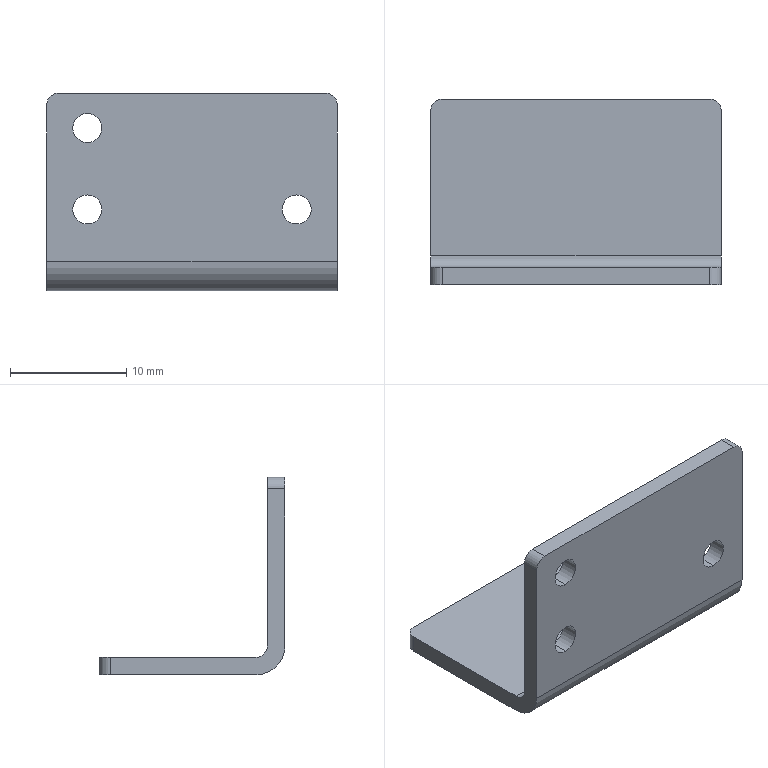Part | SolidWorks | features BaseBody 1 | 1 solid | 20 faces | box 25 x 16 x 17 mm | volume 1130 mm3 | cylinder 12 | plane 8 | commonest cylinder face diameters 2.5 x6 2 x5 5 x1
STEP:
#1=CARTESIAN_POINT('',(100.5,20.,73.25));
#2=VERTEX_POINT('',#1);
#3=CARTESIAN_POINT('',(100.5,20.,75.75));
#4=VERTEX_POINT('',#3);
#5=CARTESIAN_POINT('',(100.5,20.,74.5));
#6=DIRECTION('',(0.,1.,0.));
#7=DIRECTION('',(0.,0.,1.));
#8=AXIS2_PLACEMENT_3D('',#5,#6,#7);
#9=CIRCLE('',#8,1.25);
#10=EDGE_CURVE('',#2,#4,#9,.T.);
#11=ORIENTED_EDGE('',*,*,#10,.F.);
#12=CARTESIAN_POINT('',(100.5,21.5,73.25));
#13=VERTEX_POINT('',#12);
#14=CARTESIAN_POINT('',(100.5,46.5,73.25));
#15=DIRECTION('',(0.,1.,0.));
#16=VECTOR('',#15,1000.);
#17=LINE('',#14,#16);
#18=EDGE_CURVE('',#2,#13,#17,.T.);
#19=ORIENTED_EDGE('',*,*,#18,.T.);
#20=CARTESIAN_POINT('',(100.5,21.5,75.75));
#21=VERTEX_POINT('',#20);
#22=CARTESIAN_POINT('',(100.5,21.5,74.5));
#23=DIRECTION('',(0.,1.,0.));
#24=DIRECTION('',(0.,0.,1.));
#25=AXIS2_PLACEMENT_3D('',#22,#23,#24);
#26=CIRCLE('',#25,1.25);
#27=EDGE_CURVE('',#13,#21,#26,.T.);
#28=ORIENTED_EDGE('',*,*,#27,.T.);
#29=CARTESIAN_POINT('',(100.5,46.5,75.75));
#30=DIRECTION('',(0.,1.,0.));
#31=VECTOR('',#30,1000.);
#32=LINE('',#29,#31);
#33=EDGE_CURVE('',#4,#21,#32,.T.);
#34=ORIENTED_EDGE('',*,*,#33,.F.);
#35=EDGE_LOOP('',(#11,#19,#28,#34));
#36=FACE_OUTER_BOUND('',#35,.T.);
#37=CARTESIAN_POINT('',(100.5,46.5,74.5));
#38=DIRECTION('',(0.,1.,0.));
#39=DIRECTION('',(0.,0.,1.));
#40=AXIS2_PLACEMENT_3D('',#37,#38,#39);
#41=CYLINDRICAL_SURFACE('',#40,1.25);
#42=ADVANCED_FACE('',(#36),#41,.F.);
#43=CARTESIAN_POINT('',(118.5,20.,73.25));
#44=VERTEX_POINT('',#43);
#45=CARTESIAN_POINT('',(118.5,20.,75.75));
#46=VERTEX_POINT('',#45);
#47=CARTESIAN_POINT('',(118.5,20.,74.5));
#48=DIRECTION('',(0.,1.,0.));
#49=DIRECTION('',(0.,0.,1.));
#50=AXIS2_PLACEMENT_3D('',#47,#48,#49);
#51=CIRCLE('',#50,1.25);
#52=EDGE_CURVE('',#44,#46,#51,.T.);
#53=ORIENTED_EDGE('',*,*,#52,.F.);
#54=CARTESIAN_POINT('',(118.5,21.5,73.25));
#55=VERTEX_POINT('',#54);
#56=CARTESIAN_POINT('',(118.5,46.5,73.25));
#57=DIRECTION('',(0.,1.,0.));
#58=VECTOR('',#57,1000.);
#59=LINE('',#56,#58);
#60=EDGE_CURVE('',#44,#55,#59,.T.);
#61=ORIENTED_EDGE('',*,*,#60,.T.);
#62=CARTESIAN_POINT('',(118.5,21.5,75.75));
#63=VERTEX_POINT('',#62);
#64=CARTESIAN_POINT('',(118.5,21.5,74.5));
#65=DIRECTION('',(0.,1.,0.));
#66=DIRECTION('',(0.,0.,1.));
#67=AXIS2_PLACEMENT_3D('',#64,#65,#66);
#68=CIRCLE('',#67,1.25);
#69=EDGE_CURVE('',#55,#63,#68,.T.);
#70=ORIENTED_EDGE('',*,*,#69,.T.);
#71=CARTESIAN_POINT('',(118.5,46.5,75.75));
#72=DIRECTION('',(0.,1.,0.));
#73=VECTOR('',#72,1000.);
#74=LINE('',#71,#73);
#75=EDGE_CURVE('',#46,#63,#74,.T.);
#76=ORIENTED_EDGE('',*,*,#75,.F.);
#77=EDGE_LOOP('',(#53,#61,#70,#76));
#78=FACE_OUTER_BOUND('',#77,.T.);
#79=CARTESIAN_POINT('',(118.5,46.5,74.5));
#80=DIRECTION('',(0.,1.,0.));
#81=DIRECTION('',(0.,0.,1.));
#82=AXIS2_PLACEMENT_3D('',#79,#80,#81);
#83=CYLINDRICAL_SURFACE('',#82,1.25);
#84=ADVANCED_FACE('',(#78),#83,.F.);
#85=CARTESIAN_POINT('',(100.5,20.,80.25));
#86=VERTEX_POINT('',#85);
#87=CARTESIAN_POINT('',(100.5,20.,82.75));
#88=VERTEX_POINT('',#87);
#89=CARTESIAN_POINT('',(100.5,20.,81.5));
#90=DIRECTION('',(0.,1.,0.));
#91=DIRECTION('',(0.,0.,1.));
#92=AXIS2_PLACEMENT_3D('',#89,#90,#91);
#93=CIRCLE('',#92,1.25);
#94=EDGE_CURVE('',#86,#88,#93,.T.);
#95=ORIENTED_EDGE('',*,*,#94,.F.);
#96=CARTESIAN_POINT('',(100.5,21.5,80.25));
#97=VERTEX_POINT('',#96);
#98=CARTESIAN_POINT('',(100.5,46.5,80.25));
#99=DIRECTION('',(0.,1.,0.));
#100=VECTOR('',#99,1000.);
#101=LINE('',#98,#100);
#102=EDGE_CURVE('',#86,#97,#101,.T.);
#103=ORIENTED_EDGE('',*,*,#102,.T.);
#104=CARTESIAN_POINT('',(100.5,21.5,82.75));
#105=VERTEX_POINT('',#104);
#106=CARTESIAN_POINT('',(100.5,21.5,81.5));
#107=DIRECTION('',(0.,1.,0.));
#108=DIRECTION('',(0.,0.,1.));
#109=AXIS2_PLACEMENT_3D('',#106,#107,#108);
#110=CIRCLE('',#109,1.25);
#111=EDGE_CURVE('',#97,#105,#110,.T.);
#112=ORIENTED_EDGE('',*,*,#111,.T.);
#113=CARTESIAN_POINT('',(100.5,46.5,82.75));
#114=DIRECTION('',(0.,1.,0.));
#115=VECTOR('',#114,1000.);
#116=LINE('',#113,#115);
#117=EDGE_CURVE('',#88,#105,#116,.T.);
#118=ORIENTED_EDGE('',*,*,#117,.F.);
#119=EDGE_LOOP('',(#95,#103,#112,#118));
#120=FACE_OUTER_BOUND('',#119,.T.);
#121=CARTESIAN_POINT('',(100.5,46.5,81.5));
#122=DIRECTION('',(0.,1.,0.));
#123=DIRECTION('',(0.,0.,1.));
#124=AXIS2_PLACEMENT_3D('',#121,#122,#123);
#125=CYLINDRICAL_SURFACE('',#124,1.25);
#126=ADVANCED_FACE('',(#120),#125,.F.);
#127=CARTESIAN_POINT('',(122.,21.5,83.5));
#128=VERTEX_POINT('',#127);
#129=CARTESIAN_POINT('',(121.,21.5,84.5));
#130=VERTEX_POINT('',#129);
#131=CARTESIAN_POINT('',(121.,21.5,83.5));
#132=DIRECTION('',(0.,-1.,0.));
#133=DIRECTION('',(0.,0.,-1.));
#134=AXIS2_PLACEMENT_3D('',#131,#132,#133);
#135=CIRCLE('',#134,1.);
#136=EDGE_CURVE('',#128,#130,#135,.T.);
#137=ORIENTED_EDGE('',*,*,#136,.F.);
#138=CARTESIAN_POINT('',(122.,21.5,70.));
#139=VERTEX_POINT('',#138);
#140=CARTESIAN_POINT('',(122.,21.5,70.));
#141=DIRECTION('',(0.,0.,1.));
#142=VECTOR('',#141,1000.);
#143=LINE('',#140,#142);
#144=EDGE_CURVE('',#139,#128,#143,.T.);
#145=ORIENTED_EDGE('',*,*,#144,.F.);
#146=CARTESIAN_POINT('',(97.,21.5,70.));
#147=VERTEX_POINT('',#146);
#148=CARTESIAN_POINT('',(122.,21.5,70.));
#149=DIRECTION('',(1.,0.,0.));
#150=VECTOR('',#149,1000.);
#151=LINE('',#148,#150);
#152=EDGE_CURVE('',#147,#139,#151,.T.);
#153=ORIENTED_EDGE('',*,*,#152,.F.);
#154=CARTESIAN_POINT('',(97.,21.5,83.5));
#155=VERTEX_POINT('',#154);
#156=CARTESIAN_POINT('',(97.,21.5,70.));
#157=DIRECTION('',(0.,0.,-1.));
#158=VECTOR('',#157,1000.);
#159=LINE('',#156,#158);
#160=EDGE_CURVE('',#155,#147,#159,.T.);
#161=ORIENTED_EDGE('',*,*,#160,.F.);
#162=CARTESIAN_POINT('',(98.,21.5,84.5));
#163=VERTEX_POINT('',#162);
#164=CARTESIAN_POINT('',(98.,21.5,83.5));
#165=DIRECTION('',(0.,-1.,0.));
#166=DIRECTION('',(0.,0.,1.));
#167=AXIS2_PLACEMENT_3D('',#164,#165,#166);
#168=CIRCLE('',#167,1.);
#169=EDGE_CURVE('',#163,#155,#168,.T.);
#170=ORIENTED_EDGE('',*,*,#169,.F.);
#171=CARTESIAN_POINT('',(122.,21.5,84.5));
#172=DIRECTION('',(-1.,0.,0.));
#173=VECTOR('',#172,1000.);
#174=LINE('',#171,#173);
#175=EDGE_CURVE('',#130,#163,#174,.T.);
#176=ORIENTED_EDGE('',*,*,#175,.F.);
#177=EDGE_LOOP('',(#137,#145,#153,#161,#170,#176));
#178=FACE_OUTER_BOUND('',#177,.T.);
#179=CARTESIAN_POINT('',(100.5,21.5,74.5));
#180=DIRECTION('',(0.,1.,0.));
#181=DIRECTION('',(0.,0.,1.));
#182=AXIS2_PLACEMENT_3D('',#179,#180,#181);
#183=CIRCLE('',#182,1.25);
#184=EDGE_CURVE('',#21,#13,#183,.T.);
#185=ORIENTED_EDGE('',*,*,#184,.F.);
#186=ORIENTED_EDGE('',*,*,#27,.F.);
#187=EDGE_LOOP('',(#185,#186));
#188=FACE_BOUND('',#187,.T.);
#189=CARTESIAN_POINT('',(118.5,21.5,74.5));
#190=DIRECTION('',(0.,1.,0.));
#191=DIRECTION('',(0.,0.,1.));
#192=AXIS2_PLACEMENT_3D('',#189,#190,#191);
#193=CIRCLE('',#192,1.25);
#194=EDGE_CURVE('',#63,#55,#193,.T.);
#195=ORIENTED_EDGE('',*,*,#194,.F.);
#196=ORIENTED_EDGE('',*,*,#69,.F.);
#197=EDGE_LOOP('',(#195,#196));
#198=FACE_BOUND('',#197,.T.);
#199=CARTESIAN_POINT('',(100.5,21.5,81.5));
#200=DIRECTION('',(0.,1.,0.));
#201=DIRECTION('',(0.,0.,1.));
#202=AXIS2_PLACEMENT_3D('',#199,#200,#201);
#203=CIRCLE('',#202,1.25);
#204=EDGE_CURVE('',#105,#97,#203,.T.);
#205=ORIENTED_EDGE('',*,*,#204,.F.);
#206=ORIENTED_EDGE('',*,*,#111,.F.);
#207=EDGE_LOOP('',(#205,#206));
#208=FACE_BOUND('',#207,.T.);
#209=CARTESIAN_POINT('',(122.,21.5,70.));
#210=DIRECTION('',(0.,-1.,0.));
#211=DIRECTION('',(0.,0.,-1.));
#212=AXIS2_PLACEMENT_3D('',#209,#210,#211);
#213=PLANE('',#212);
#214=ADVANCED_FACE('',(#178,#188,#198,#208),#213,.F.);
#215=CARTESIAN_POINT('',(121.,20.,84.5));
#216=VERTEX_POINT('',#215);
#217=CARTESIAN_POINT('',(121.,21.5,84.5));
#218=DIRECTION('',(0.,-1.,0.));
#219=VECTOR('',#218,1000.);
#220=LINE('',#217,#219);
#221=EDGE_CURVE('',#130,#216,#220,.T.);
#222=ORIENTED_EDGE('',*,*,#221,.F.);
#223=ORIENTED_EDGE('',*,*,#175,.T.);
#224=CARTESIAN_POINT('',(98.,20.,84.5));
#225=VERTEX_POINT('',#224);
#226=CARTESIAN_POINT('',(98.,21.5,84.5));
#227=DIRECTION('',(0.,1.,0.));
#228=VECTOR('',#227,1000.);
#229=LINE('',#226,#228);
#230=EDGE_CURVE('',#225,#163,#229,.T.);
#231=ORIENTED_EDGE('',*,*,#230,.F.);
#232=CARTESIAN_POINT('',(122.,20.,84.5));
#233=DIRECTION('',(-1.,0.,0.));
#234=VECTOR('',#233,1000.);
#235=LINE('',#232,#234);
#236=EDGE_CURVE('',#216,#225,#235,.T.);
#237=ORIENTED_EDGE('',*,*,#236,.F.);
#238=EDGE_LOOP('',(#222,#223,#231,#237));
#239=FACE_OUTER_BOUND('',#238,.T.);
#240=CARTESIAN_POINT('',(122.,21.5,84.5));
#241=DIRECTION('',(0.,0.,-1.));
#242=DIRECTION('',(-1.,0.,0.));
#243=AXIS2_PLACEMENT_3D('',#240,#241,#242);
#244=PLANE('',#243);
#245=ADVANCED_FACE('',(#239),#244,.F.);
#246=CARTESIAN_POINT('',(122.,20.,83.5));
#247=VERTEX_POINT('',#246);
#248=CARTESIAN_POINT('',(121.,20.,83.5));
#249=DIRECTION('',(0.,1.,0.));
#250=DIRECTION('',(0.,0.,-1.));
#251=AXIS2_PLACEMENT_3D('',#248,#249,#250);
#252=CIRCLE('',#251,1.);
#253=EDGE_CURVE('',#216,#247,#252,.T.);
#254=ORIENTED_EDGE('',*,*,#253,.T.);
#255=CARTESIAN_POINT('',(122.,22.5,83.5));
#256=DIRECTION('',(0.,1.,0.));
#257=VECTOR('',#256,1000.);
#258=LINE('',#255,#257);
#259=EDGE_CURVE('',#247,#128,#258,.T.);
#260=ORIENTED_EDGE('',*,*,#259,.T.);
#261=ORIENTED_EDGE('',*,*,#136,.T.);
#262=ORIENTED_EDGE('',*,*,#221,.T.);
#263=EDGE_LOOP('',(#254,#260,#261,#262));
#264=FACE_OUTER_BOUND('',#263,.T.);
#265=CARTESIAN_POINT('',(121.,22.5,83.5));
#266=DIRECTION('',(0.,-1.,0.));
#267=DIRECTION('',(0.,0.,-1.));
#268=AXIS2_PLACEMENT_3D('',#265,#266,#267);
#269=CYLINDRICAL_SURFACE('',#268,1.);
#270=ADVANCED_FACE('',(#264),#269,.T.);
#271=CARTESIAN_POINT('',(122.,35.,69.));
#272=VERTEX_POINT('',#271);
#273=CARTESIAN_POINT('',(122.,22.5,69.));
#274=VERTEX_POINT('',#273);
#275=CARTESIAN_POINT('',(122.,22.5,69.));
#276=DIRECTION('',(0.,-1.,0.));
#277=VECTOR('',#276,1000.);
#278=LINE('',#275,#277);
#279=EDGE_CURVE('',#272,#274,#278,.T.);
#280=ORIENTED_EDGE('',*,*,#279,.T.);
#281=CARTESIAN_POINT('',(122.,22.5,70.));
#282=DIRECTION('',(-1.,0.,0.));
#283=DIRECTION('',(0.,0.,-1.));
#284=AXIS2_PLACEMENT_3D('',#281,#282,#283);
#285=CIRCLE('',#284,1.);
#286=EDGE_CURVE('',#274,#139,#285,.T.);
#287=ORIENTED_EDGE('',*,*,#286,.T.);
#288=ORIENTED_EDGE('',*,*,#144,.T.);
#289=ORIENTED_EDGE('',*,*,#259,.F.);
#290=CARTESIAN_POINT('',(122.,20.,70.));
#291=VERTEX_POINT('',#290);
#292=CARTESIAN_POINT('',(122.,20.,70.));
#293=DIRECTION('',(0.,0.,-1.));
#294=VECTOR('',#293,1000.);
#295=LINE('',#292,#294);
#296=EDGE_CURVE('',#247,#291,#295,.T.);
#297=ORIENTED_EDGE('',*,*,#296,.T.);
#298=CARTESIAN_POINT('',(122.,22.5,67.5));
#299=VERTEX_POINT('',#298);
#300=CARTESIAN_POINT('',(122.,22.5,70.));
#301=DIRECTION('',(1.,0.,0.));
#302=DIRECTION('',(0.,0.,-1.));
#303=AXIS2_PLACEMENT_3D('',#300,#301,#302);
#304=CIRCLE('',#303,2.5);
#305=EDGE_CURVE('',#291,#299,#304,.T.);
#306=ORIENTED_EDGE('',*,*,#305,.T.);
#307=CARTESIAN_POINT('',(122.,35.,67.5));
#308=VERTEX_POINT('',#307);
#309=CARTESIAN_POINT('',(122.,22.5,67.5));
#310=DIRECTION('',(0.,1.,0.));
#311=VECTOR('',#310,1000.);
#312=LINE('',#309,#311);
#313=EDGE_CURVE('',#299,#308,#312,.T.);
#314=ORIENTED_EDGE('',*,*,#313,.T.);
#315=CARTESIAN_POINT('',(122.,35.,70.));
#316=DIRECTION('',(0.,0.,1.));
#317=VECTOR('',#316,1000.);
#318=LINE('',#315,#317);
#319=EDGE_CURVE('',#308,#272,#318,.T.);
#320=ORIENTED_EDGE('',*,*,#319,.T.);
#321=EDGE_LOOP('',(#280,#287,#288,#289,#297,#306,#314,#320));
#322=FACE_OUTER_BOUND('',#321,.T.);
#323=CARTESIAN_POINT('',(122.,22.5,70.));
#324=DIRECTION('',(1.,0.,0.));
#325=DIRECTION('',(0.,0.,-1.));
#326=AXIS2_PLACEMENT_3D('',#323,#324,#325);
#327=PLANE('',#326);
#328=ADVANCED_FACE('',(#322),#327,.T.);
#329=ORIENTED_EDGE('',*,*,#152,.T.);
#330=ORIENTED_EDGE('',*,*,#286,.F.);
#331=CARTESIAN_POINT('',(97.,22.5,69.));
#332=VERTEX_POINT('',#331);
#333=CARTESIAN_POINT('',(122.,22.5,69.));
#334=DIRECTION('',(1.,0.,0.));
#335=VECTOR('',#334,1000.);
#336=LINE('',#333,#335);
#337=EDGE_CURVE('',#332,#274,#336,.T.);
#338=ORIENTED_EDGE('',*,*,#337,.F.);
#339=CARTESIAN_POINT('',(97.,22.5,70.));
#340=DIRECTION('',(1.,0.,0.));
#341=DIRECTION('',(0.,0.,-1.));
#342=AXIS2_PLACEMENT_3D('',#339,#340,#341);
#343=CIRCLE('',#342,1.);
#344=EDGE_CURVE('',#147,#332,#343,.T.);
#345=ORIENTED_EDGE('',*,*,#344,.F.);
#346=EDGE_LOOP('',(#329,#330,#338,#345));
#347=FACE_OUTER_BOUND('',#346,.T.);
#348=CARTESIAN_POINT('',(122.,22.5,70.));
#349=DIRECTION('',(1.,0.,0.));
#350=DIRECTION('',(0.,0.,-1.));
#351=AXIS2_PLACEMENT_3D('',#348,#349,#350);
#352=CYLINDRICAL_SURFACE('',#351,1.);
#353=ADVANCED_FACE('',(#347),#352,.F.);
#354=CARTESIAN_POINT('',(97.,20.,83.5));
#355=VERTEX_POINT('',#354);
#356=CARTESIAN_POINT('',(97.,22.5,83.5));
#357=DIRECTION('',(0.,-1.,0.));
#358=VECTOR('',#357,1000.);
#359=LINE('',#356,#358);
#360=EDGE_CURVE('',#155,#355,#359,.T.);
#361=ORIENTED_EDGE('',*,*,#360,.F.);
#362=ORIENTED_EDGE('',*,*,#160,.T.);
#363=ORIENTED_EDGE('',*,*,#344,.T.);
#364=CARTESIAN_POINT('',(97.,35.,69.));
#365=VERTEX_POINT('',#364);
#366=CARTESIAN_POINT('',(97.,22.5,69.));
#367=DIRECTION('',(0.,-1.,0.));
#368=VECTOR('',#367,1000.);
#369=LINE('',#366,#368);
#370=EDGE_CURVE('',#365,#332,#369,.T.);
#371=ORIENTED_EDGE('',*,*,#370,.F.);
#372=CARTESIAN_POINT('',(97.,35.,67.5));
#373=VERTEX_POINT('',#372);
#374=CARTESIAN_POINT('',(97.,35.,70.));
#375=DIRECTION('',(0.,0.,1.));
#376=VECTOR('',#375,1000.);
#377=LINE('',#374,#376);
#378=EDGE_CURVE('',#373,#365,#377,.T.);
#379=ORIENTED_EDGE('',*,*,#378,.F.);
#380=CARTESIAN_POINT('',(97.,22.5,67.5));
#381=VERTEX_POINT('',#380);
#382=CARTESIAN_POINT('',(97.,22.5,67.5));
#383=DIRECTION('',(0.,1.,0.));
#384=VECTOR('',#383,1000.);
#385=LINE('',#382,#384);
#386=EDGE_CURVE('',#381,#373,#385,.T.);
#387=ORIENTED_EDGE('',*,*,#386,.F.);
#388=CARTESIAN_POINT('',(97.,20.,70.));
#389=VERTEX_POINT('',#388);
#390=CARTESIAN_POINT('',(97.,22.5,70.));
#391=DIRECTION('',(1.,0.,0.));
#392=DIRECTION('',(0.,0.,-1.));
#393=AXIS2_PLACEMENT_3D('',#390,#391,#392);
#394=CIRCLE('',#393,2.5);
#395=EDGE_CURVE('',#389,#381,#394,.T.);
#396=ORIENTED_EDGE('',*,*,#395,.F.);
#397=CARTESIAN_POINT('',(97.,20.,70.));
#398=DIRECTION('',(0.,0.,-1.));
#399=VECTOR('',#398,1000.);
#400=LINE('',#397,#399);
#401=EDGE_CURVE('',#355,#389,#400,.T.);
#402=ORIENTED_EDGE('',*,*,#401,.F.);
#403=EDGE_LOOP('',(#361,#362,#363,#371,#379,#387,#396,#402));
#404=FACE_OUTER_BOUND('',#403,.T.);
#405=CARTESIAN_POINT('',(97.,22.5,70.));
#406=DIRECTION('',(1.,0.,0.));
#407=DIRECTION('',(0.,0.,-1.));
#408=AXIS2_PLACEMENT_3D('',#405,#406,#407);
#409=PLANE('',#408);
#410=ADVANCED_FACE('',(#404),#409,.F.);
#411=CARTESIAN_POINT('',(98.,20.,83.5));
#412=DIRECTION('',(0.,1.,0.));
#413=DIRECTION('',(0.,0.,1.));
#414=AXIS2_PLACEMENT_3D('',#411,#412,#413);
#415=CIRCLE('',#414,1.);
#416=EDGE_CURVE('',#355,#225,#415,.T.);
#417=ORIENTED_EDGE('',*,*,#416,.T.);
#418=ORIENTED_EDGE('',*,*,#230,.T.);
#419=ORIENTED_EDGE('',*,*,#169,.T.);
#420=ORIENTED_EDGE('',*,*,#360,.T.);
#421=EDGE_LOOP('',(#417,#418,#419,#420));
#422=FACE_OUTER_BOUND('',#421,.T.);
#423=CARTESIAN_POINT('',(98.,21.5,83.5));
#424=DIRECTION('',(0.,1.,0.));
#425=DIRECTION('',(0.,0.,1.));
#426=AXIS2_PLACEMENT_3D('',#423,#424,#425);
#427=CYLINDRICAL_SURFACE('',#426,1.);
#428=ADVANCED_FACE('',(#422),#427,.T.);
#429=ORIENTED_EDGE('',*,*,#18,.F.);
#430=CARTESIAN_POINT('',(100.5,20.,74.5));
#431=DIRECTION('',(0.,1.,0.));
#432=DIRECTION('',(0.,0.,1.));
#433=AXIS2_PLACEMENT_3D('',#430,#431,#432);
#434=CIRCLE('',#433,1.25);
#435=EDGE_CURVE('',#4,#2,#434,.T.);
#436=ORIENTED_EDGE('',*,*,#435,.F.);
#437=ORIENTED_EDGE('',*,*,#33,.T.);
#438=ORIENTED_EDGE('',*,*,#184,.T.);
#439=EDGE_LOOP('',(#429,#436,#437,#438));
#440=FACE_OUTER_BOUND('',#439,.T.);
#441=CARTESIAN_POINT('',(100.5,46.5,74.5));
#442=DIRECTION('',(0.,1.,0.));
#443=DIRECTION('',(0.,0.,1.));
#444=AXIS2_PLACEMENT_3D('',#441,#442,#443);
#445=CYLINDRICAL_SURFACE('',#444,1.25);
#446=ADVANCED_FACE('',(#440),#445,.F.);
#447=ORIENTED_EDGE('',*,*,#60,.F.);
#448=CARTESIAN_POINT('',(118.5,20.,74.5));
#449=DIRECTION('',(0.,1.,0.));
#450=DIRECTION('',(0.,0.,1.));
#451=AXIS2_PLACEMENT_3D('',#448,#449,#450);
#452=CIRCLE('',#451,1.25);
#453=EDGE_CURVE('',#46,#44,#452,.T.);
#454=ORIENTED_EDGE('',*,*,#453,.F.);
#455=ORIENTED_EDGE('',*,*,#75,.T.);
#456=ORIENTED_EDGE('',*,*,#194,.T.);
#457=EDGE_LOOP('',(#447,#454,#455,#456));
#458=FACE_OUTER_BOUND('',#457,.T.);
#459=CARTESIAN_POINT('',(118.5,46.5,74.5));
#460=DIRECTION('',(0.,1.,0.));
#461=DIRECTION('',(0.,0.,1.));
#462=AXIS2_PLACEMENT_3D('',#459,#460,#461);
#463=CYLINDRICAL_SURFACE('',#462,1.25);
#464=ADVANCED_FACE('',(#458),#463,.F.);
#465=ORIENTED_EDGE('',*,*,#102,.F.);
#466=CARTESIAN_POINT('',(100.5,20.,81.5));
#467=DIRECTION('',(0.,1.,0.));
#468=DIRECTION('',(0.,0.,1.));
#469=AXIS2_PLACEMENT_3D('',#466,#467,#468);
#470=CIRCLE('',#469,1.25);
#471=EDGE_CURVE('',#88,#86,#470,.T.);
#472=ORIENTED_EDGE('',*,*,#471,.F.);
#473=ORIENTED_EDGE('',*,*,#117,.T.);
#474=ORIENTED_EDGE('',*,*,#204,.T.);
#475=EDGE_LOOP('',(#465,#472,#473,#474));
#476=FACE_OUTER_BOUND('',#475,.T.);
#477=CARTESIAN_POINT('',(100.5,46.5,81.5));
#478=DIRECTION('',(0.,1.,0.));
#479=DIRECTION('',(0.,0.,1.));
#480=AXIS2_PLACEMENT_3D('',#477,#478,#479);
#481=CYLINDRICAL_SURFACE('',#480,1.25);
#482=ADVANCED_FACE('',(#476),#481,.F.);
#483=ORIENTED_EDGE('',*,*,#253,.F.);
#484=ORIENTED_EDGE('',*,*,#236,.T.);
#485=ORIENTED_EDGE('',*,*,#416,.F.);
#486=ORIENTED_EDGE('',*,*,#401,.T.);
#487=CARTESIAN_POINT('',(122.,20.,70.));
#488=DIRECTION('',(-1.,0.,0.));
#489=VECTOR('',#488,1000.);
#490=LINE('',#487,#489);
#491=EDGE_CURVE('',#291,#389,#490,.T.);
#492=ORIENTED_EDGE('',*,*,#491,.F.);
#493=ORIENTED_EDGE('',*,*,#296,.F.);
#494=EDGE_LOOP('',(#483,#484,#485,#486,#492,#493));
#495=FACE_OUTER_BOUND('',#494,.T.);
#496=ORIENTED_EDGE('',*,*,#435,.T.);
#497=ORIENTED_EDGE('',*,*,#10,.T.);
#498=EDGE_LOOP('',(#496,#497));
#499=FACE_BOUND('',#498,.T.);
#500=ORIENTED_EDGE('',*,*,#453,.T.);
#501=ORIENTED_EDGE('',*,*,#52,.T.);
#502=EDGE_LOOP('',(#500,#501));
#503=FACE_BOUND('',#502,.T.);
#504=ORIENTED_EDGE('',*,*,#471,.T.);
#505=ORIENTED_EDGE('',*,*,#94,.T.);
#506=EDGE_LOOP('',(#504,#505));
#507=FACE_BOUND('',#506,.T.);
#508=CARTESIAN_POINT('',(122.,20.,84.5));
#509=DIRECTION('',(0.,1.,0.));
#510=DIRECTION('',(0.,0.,1.));
#511=AXIS2_PLACEMENT_3D('',#508,#509,#510);
#512=PLANE('',#511);
#513=ADVANCED_FACE('',(#495,#499,#503,#507),#512,.F.);
#514=CARTESIAN_POINT('',(121.,36.,69.));
#515=VERTEX_POINT('',#514);
#516=CARTESIAN_POINT('',(121.,35.,69.));
#517=DIRECTION('',(0.,0.,-1.));
#518=DIRECTION('',(1.,0.,0.));
#519=AXIS2_PLACEMENT_3D('',#516,#517,#518);
#520=CIRCLE('',#519,1.);
#521=EDGE_CURVE('',#515,#272,#520,.T.);
#522=ORIENTED_EDGE('',*,*,#521,.F.);
#523=CARTESIAN_POINT('',(98.,36.,69.));
#524=VERTEX_POINT('',#523);
#525=CARTESIAN_POINT('',(122.,36.,69.));
#526=DIRECTION('',(1.,0.,0.));
#527=VECTOR('',#526,1000.);
#528=LINE('',#525,#527);
#529=EDGE_CURVE('',#524,#515,#528,.T.);
#530=ORIENTED_EDGE('',*,*,#529,.F.);
#531=CARTESIAN_POINT('',(98.,35.,69.));
#532=DIRECTION('',(0.,0.,-1.));
#533=DIRECTION('',(-1.,0.,0.));
#534=AXIS2_PLACEMENT_3D('',#531,#532,#533);
#535=CIRCLE('',#534,1.);
#536=EDGE_CURVE('',#365,#524,#535,.T.);
#537=ORIENTED_EDGE('',*,*,#536,.F.);
#538=ORIENTED_EDGE('',*,*,#370,.T.);
#539=ORIENTED_EDGE('',*,*,#337,.T.);
#540=ORIENTED_EDGE('',*,*,#279,.F.);
#541=EDGE_LOOP('',(#522,#530,#537,#538,#539,#540));
#542=FACE_OUTER_BOUND('',#541,.T.);
#543=CARTESIAN_POINT('',(122.,36.,69.));
#544=DIRECTION('',(0.,0.,-1.));
#545=DIRECTION('',(-1.,0.,0.));
#546=AXIS2_PLACEMENT_3D('',#543,#544,#545);
#547=PLANE('',#546);
#548=ADVANCED_FACE('',(#542),#547,.F.);
#549=ORIENTED_EDGE('',*,*,#521,.T.);
#550=ORIENTED_EDGE('',*,*,#319,.F.);
#551=CARTESIAN_POINT('',(121.,36.,67.5));
#552=VERTEX_POINT('',#551);
#553=CARTESIAN_POINT('',(121.,35.,67.5));
#554=DIRECTION('',(0.,0.,1.));
#555=DIRECTION('',(1.,0.,0.));
#556=AXIS2_PLACEMENT_3D('',#553,#554,#555);
#557=CIRCLE('',#556,1.);
#558=EDGE_CURVE('',#308,#552,#557,.T.);
#559=ORIENTED_EDGE('',*,*,#558,.T.);
#560=CARTESIAN_POINT('',(121.,36.,70.));
#561=DIRECTION('',(0.,0.,1.));
#562=VECTOR('',#561,1000.);
#563=LINE('',#560,#562);
#564=EDGE_CURVE('',#552,#515,#563,.T.);
#565=ORIENTED_EDGE('',*,*,#564,.T.);
#566=EDGE_LOOP('',(#549,#550,#559,#565));
#567=FACE_OUTER_BOUND('',#566,.T.);
#568=CARTESIAN_POINT('',(121.,35.,70.));
#569=DIRECTION('',(0.,0.,1.));
#570=DIRECTION('',(1.,0.,0.));
#571=AXIS2_PLACEMENT_3D('',#568,#569,#570);
#572=CYLINDRICAL_SURFACE('',#571,1.);
#573=ADVANCED_FACE('',(#567),#572,.T.);
#574=ORIENTED_EDGE('',*,*,#558,.F.);
#575=ORIENTED_EDGE('',*,*,#313,.F.);
#576=CARTESIAN_POINT('',(122.,22.5,67.5));
#577=DIRECTION('',(1.,0.,0.));
#578=VECTOR('',#577,1000.);
#579=LINE('',#576,#578);
#580=EDGE_CURVE('',#381,#299,#579,.T.);
#581=ORIENTED_EDGE('',*,*,#580,.F.);
#582=ORIENTED_EDGE('',*,*,#386,.T.);
#583=CARTESIAN_POINT('',(98.,36.,67.5));
#584=VERTEX_POINT('',#583);
#585=CARTESIAN_POINT('',(98.,35.,67.5));
#586=DIRECTION('',(0.,0.,1.));
#587=DIRECTION('',(-1.,0.,0.));
#588=AXIS2_PLACEMENT_3D('',#585,#586,#587);
#589=CIRCLE('',#588,1.);
#590=EDGE_CURVE('',#584,#373,#589,.T.);
#591=ORIENTED_EDGE('',*,*,#590,.F.);
#592=CARTESIAN_POINT('',(122.,36.,67.5));
#593=DIRECTION('',(-1.,0.,0.));
#594=VECTOR('',#593,1000.);
#595=LINE('',#592,#594);
#596=EDGE_CURVE('',#552,#584,#595,.T.);
#597=ORIENTED_EDGE('',*,*,#596,.F.);
#598=EDGE_LOOP('',(#574,#575,#581,#582,#591,#597));
#599=FACE_OUTER_BOUND('',#598,.T.);
#600=CARTESIAN_POINT('',(122.,22.5,67.5));
#601=DIRECTION('',(0.,0.,1.));
#602=DIRECTION('',(1.,0.,0.));
#603=AXIS2_PLACEMENT_3D('',#600,#601,#602);
#604=PLANE('',#603);
#605=ADVANCED_FACE('',(#599),#604,.F.);
#606=ORIENTED_EDGE('',*,*,#305,.F.);
#607=ORIENTED_EDGE('',*,*,#491,.T.);
#608=ORIENTED_EDGE('',*,*,#395,.T.);
#609=ORIENTED_EDGE('',*,*,#580,.T.);
#610=EDGE_LOOP('',(#606,#607,#608,#609));
#611=FACE_OUTER_BOUND('',#610,.T.);
#612=CARTESIAN_POINT('',(122.,22.5,70.));
#613=DIRECTION('',(1.,0.,0.));
#614=DIRECTION('',(0.,0.,-1.));
#615=AXIS2_PLACEMENT_3D('',#612,#613,#614);
#616=CYLINDRICAL_SURFACE('',#615,2.5);
#617=ADVANCED_FACE('',(#611),#616,.T.);
#618=ORIENTED_EDGE('',*,*,#536,.T.);
#619=CARTESIAN_POINT('',(98.,36.,67.5));
#620=DIRECTION('',(0.,0.,-1.));
#621=VECTOR('',#620,1000.);
#622=LINE('',#619,#621);
#623=EDGE_CURVE('',#524,#584,#622,.T.);
#624=ORIENTED_EDGE('',*,*,#623,.T.);
#625=ORIENTED_EDGE('',*,*,#590,.T.);
#626=ORIENTED_EDGE('',*,*,#378,.T.);
#627=EDGE_LOOP('',(#618,#624,#625,#626));
#628=FACE_OUTER_BOUND('',#627,.T.);
#629=CARTESIAN_POINT('',(98.,35.,67.5));
#630=DIRECTION('',(0.,0.,-1.));
#631=DIRECTION('',(-1.,0.,0.));
#632=AXIS2_PLACEMENT_3D('',#629,#630,#631);
#633=CYLINDRICAL_SURFACE('',#632,1.);
#634=ADVANCED_FACE('',(#628),#633,.T.);
#635=ORIENTED_EDGE('',*,*,#564,.F.);
#636=ORIENTED_EDGE('',*,*,#596,.T.);
#637=ORIENTED_EDGE('',*,*,#623,.F.);
#638=ORIENTED_EDGE('',*,*,#529,.T.);
#639=EDGE_LOOP('',(#635,#636,#637,#638));
#640=FACE_OUTER_BOUND('',#639,.T.);
#641=CARTESIAN_POINT('',(122.,36.,67.5));
#642=DIRECTION('',(0.,-1.,0.));
#643=DIRECTION('',(0.,0.,-1.));
#644=AXIS2_PLACEMENT_3D('',#641,#642,#643);
#645=PLANE('',#644);
#646=ADVANCED_FACE('',(#640),#645,.F.);
#647=CLOSED_SHELL('',(#42,#84,#126,#214,#245,#270,#328,#353,#410,#428,#446,#464,#482,#513,#548,#573,#605,#617,#634,#646));
#648=MANIFOLD_SOLID_BREP('',#647);
#649=CARTESIAN_POINT('',(0.,0.,0.));
#650=DIRECTION('',(0.,0.,1.));
#651=DIRECTION('',(1.,0.,0.));
#652=AXIS2_PLACEMENT_3D('',#649,#650,#651);
#653=(LENGTH_UNIT()NAMED_UNIT(*)SI_UNIT(.MILLI.,.METRE.));
#654=UNCERTAINTY_MEASURE_WITH_UNIT(LENGTH_MEASURE(0.00001),#653,'','');
#655=(NAMED_UNIT(*)PLANE_ANGLE_UNIT()SI_UNIT($,.RADIAN.));
#656=(NAMED_UNIT(*)SI_UNIT($,.STERADIAN.)SOLID_ANGLE_UNIT());
#657=(GEOMETRIC_REPRESENTATION_CONTEXT(3)GLOBAL_UNCERTAINTY_ASSIGNED_CONTEXT((#654))GLOBAL_UNIT_ASSIGNED_CONTEXT((#653,#655,#656))REPRESENTATION_CONTEXT('',''));
#658=ADVANCED_BREP_SHAPE_REPRESENTATION('',(#648,#652),#657);